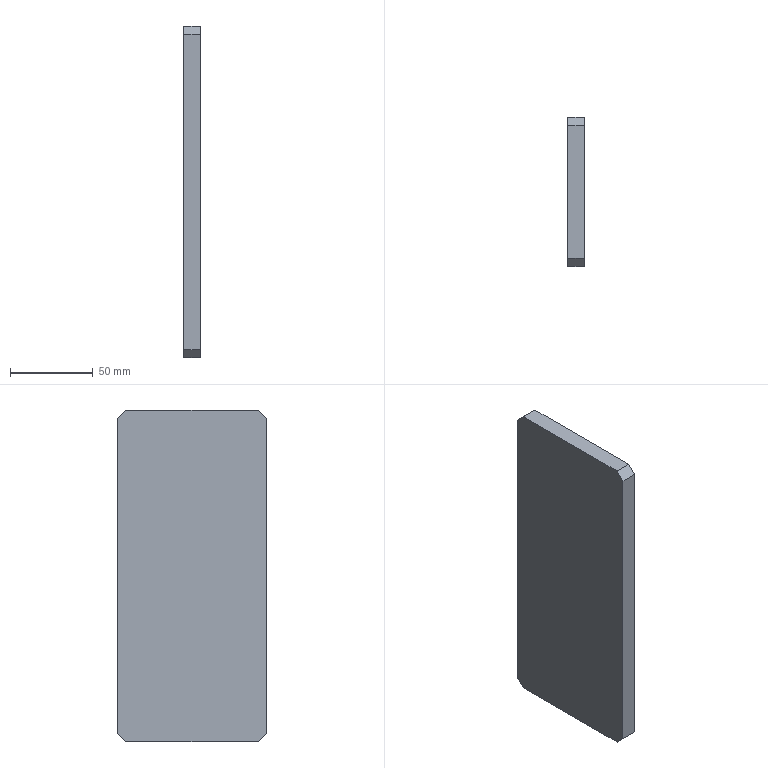Part | SolidWorks | features BaseBody 1 | 1 solid | 10 faces | box 10 x 90 x 200 mm | volume 179500 mm3 | plane 10
STEP:
#1=CARTESIAN_POINT('',(0.,5.,0.));
#2=VERTEX_POINT('',#1);
#3=CARTESIAN_POINT('',(0.,85.,0.));
#4=VERTEX_POINT('',#3);
#5=CARTESIAN_POINT('',(0.,0.,0.));
#6=DIRECTION('',(0.,1.,0.));
#7=VECTOR('',#6,1000.);
#8=LINE('',#5,#7);
#9=EDGE_CURVE('',#2,#4,#8,.T.);
#10=ORIENTED_EDGE('',*,*,#9,.T.);
#11=CARTESIAN_POINT('',(0.,90.,-5.));
#12=VERTEX_POINT('',#11);
#13=CARTESIAN_POINT('',(0.,85.,0.));
#14=DIRECTION('',(0.,0.7071,-0.7071));
#15=VECTOR('',#14,1000.);
#16=LINE('',#13,#15);
#17=EDGE_CURVE('',#4,#12,#16,.T.);
#18=ORIENTED_EDGE('',*,*,#17,.T.);
#19=CARTESIAN_POINT('',(0.,90.,-195.));
#20=VERTEX_POINT('',#19);
#21=CARTESIAN_POINT('',(0.,90.,0.));
#22=DIRECTION('',(0.,0.,-1.));
#23=VECTOR('',#22,1000.);
#24=LINE('',#21,#23);
#25=EDGE_CURVE('',#12,#20,#24,.T.);
#26=ORIENTED_EDGE('',*,*,#25,.T.);
#27=CARTESIAN_POINT('',(0.,85.,-200.));
#28=VERTEX_POINT('',#27);
#29=CARTESIAN_POINT('',(0.,90.,-195.));
#30=DIRECTION('',(0.,-0.7071,-0.7071));
#31=VECTOR('',#30,1000.);
#32=LINE('',#29,#31);
#33=EDGE_CURVE('',#20,#28,#32,.T.);
#34=ORIENTED_EDGE('',*,*,#33,.T.);
#35=CARTESIAN_POINT('',(0.,5.,-200.));
#36=VERTEX_POINT('',#35);
#37=CARTESIAN_POINT('',(0.,0.,-200.));
#38=DIRECTION('',(0.,-1.,0.));
#39=VECTOR('',#38,1000.);
#40=LINE('',#37,#39);
#41=EDGE_CURVE('',#28,#36,#40,.T.);
#42=ORIENTED_EDGE('',*,*,#41,.T.);
#43=CARTESIAN_POINT('',(0.,0.,-195.));
#44=VERTEX_POINT('',#43);
#45=CARTESIAN_POINT('',(0.,5.,-200.));
#46=DIRECTION('',(0.,-0.7071,0.7071));
#47=VECTOR('',#46,1000.);
#48=LINE('',#45,#47);
#49=EDGE_CURVE('',#36,#44,#48,.T.);
#50=ORIENTED_EDGE('',*,*,#49,.T.);
#51=CARTESIAN_POINT('',(0.,0.,-5.));
#52=VERTEX_POINT('',#51);
#53=CARTESIAN_POINT('',(0.,0.,0.));
#54=DIRECTION('',(0.,0.,1.));
#55=VECTOR('',#54,1000.);
#56=LINE('',#53,#55);
#57=EDGE_CURVE('',#44,#52,#56,.T.);
#58=ORIENTED_EDGE('',*,*,#57,.T.);
#59=CARTESIAN_POINT('',(0.,0.,-5.));
#60=DIRECTION('',(0.,0.7071,0.7071));
#61=VECTOR('',#60,1000.);
#62=LINE('',#59,#61);
#63=EDGE_CURVE('',#52,#2,#62,.T.);
#64=ORIENTED_EDGE('',*,*,#63,.T.);
#65=EDGE_LOOP('',(#10,#18,#26,#34,#42,#50,#58,#64));
#66=FACE_OUTER_BOUND('',#65,.T.);
#67=CARTESIAN_POINT('',(0.,0.,0.));
#68=DIRECTION('',(-1.,0.,0.));
#69=DIRECTION('',(0.,0.,1.));
#70=AXIS2_PLACEMENT_3D('',#67,#68,#69);
#71=PLANE('',#70);
#72=ADVANCED_FACE('',(#66),#71,.T.);
#73=CARTESIAN_POINT('',(10.,90.,-5.));
#74=VERTEX_POINT('',#73);
#75=CARTESIAN_POINT('',(10.,90.,-5.));
#76=DIRECTION('',(1.,0.,0.));
#77=VECTOR('',#76,1000.);
#78=LINE('',#75,#77);
#79=EDGE_CURVE('',#12,#74,#78,.T.);
#80=ORIENTED_EDGE('',*,*,#79,.F.);
#81=ORIENTED_EDGE('',*,*,#17,.F.);
#82=CARTESIAN_POINT('',(10.,85.,0.));
#83=VERTEX_POINT('',#82);
#84=CARTESIAN_POINT('',(10.,85.,0.));
#85=DIRECTION('',(-1.,0.,0.));
#86=VECTOR('',#85,1000.);
#87=LINE('',#84,#86);
#88=EDGE_CURVE('',#83,#4,#87,.T.);
#89=ORIENTED_EDGE('',*,*,#88,.F.);
#90=CARTESIAN_POINT('',(10.,85.,0.));
#91=DIRECTION('',(0.,-0.7071,0.7071));
#92=VECTOR('',#91,1000.);
#93=LINE('',#90,#92);
#94=EDGE_CURVE('',#74,#83,#93,.T.);
#95=ORIENTED_EDGE('',*,*,#94,.F.);
#96=EDGE_LOOP('',(#80,#81,#89,#95));
#97=FACE_OUTER_BOUND('',#96,.T.);
#98=CARTESIAN_POINT('',(10.,85.,0.));
#99=DIRECTION('',(0.,-0.7071,-0.7071));
#100=DIRECTION('',(0.,0.7071,-0.7071));
#101=AXIS2_PLACEMENT_3D('',#98,#99,#100);
#102=PLANE('',#101);
#103=ADVANCED_FACE('',(#97),#102,.F.);
#104=CARTESIAN_POINT('',(10.,5.,0.));
#105=VERTEX_POINT('',#104);
#106=CARTESIAN_POINT('',(10.,5.,0.));
#107=DIRECTION('',(-1.,0.,0.));
#108=VECTOR('',#107,1000.);
#109=LINE('',#106,#108);
#110=EDGE_CURVE('',#105,#2,#109,.T.);
#111=ORIENTED_EDGE('',*,*,#110,.F.);
#112=CARTESIAN_POINT('',(10.,0.,0.));
#113=DIRECTION('',(0.,-1.,0.));
#114=VECTOR('',#113,1000.);
#115=LINE('',#112,#114);
#116=EDGE_CURVE('',#83,#105,#115,.T.);
#117=ORIENTED_EDGE('',*,*,#116,.F.);
#118=ORIENTED_EDGE('',*,*,#88,.T.);
#119=ORIENTED_EDGE('',*,*,#9,.F.);
#120=EDGE_LOOP('',(#111,#117,#118,#119));
#121=FACE_OUTER_BOUND('',#120,.T.);
#122=CARTESIAN_POINT('',(10.,0.,0.));
#123=DIRECTION('',(0.,0.,-1.));
#124=DIRECTION('',(0.,1.,0.));
#125=AXIS2_PLACEMENT_3D('',#122,#123,#124);
#126=PLANE('',#125);
#127=ADVANCED_FACE('',(#121),#126,.F.);
#128=ORIENTED_EDGE('',*,*,#110,.T.);
#129=ORIENTED_EDGE('',*,*,#63,.F.);
#130=CARTESIAN_POINT('',(10.,0.,-5.));
#131=VERTEX_POINT('',#130);
#132=CARTESIAN_POINT('',(10.,0.,-5.));
#133=DIRECTION('',(-1.,0.,0.));
#134=VECTOR('',#133,1000.);
#135=LINE('',#132,#134);
#136=EDGE_CURVE('',#131,#52,#135,.T.);
#137=ORIENTED_EDGE('',*,*,#136,.F.);
#138=CARTESIAN_POINT('',(10.,0.,-5.));
#139=DIRECTION('',(0.,-0.7071,-0.7071));
#140=VECTOR('',#139,1000.);
#141=LINE('',#138,#140);
#142=EDGE_CURVE('',#105,#131,#141,.T.);
#143=ORIENTED_EDGE('',*,*,#142,.F.);
#144=EDGE_LOOP('',(#128,#129,#137,#143));
#145=FACE_OUTER_BOUND('',#144,.T.);
#146=CARTESIAN_POINT('',(10.,0.,-5.));
#147=DIRECTION('',(0.,0.7071,-0.7071));
#148=DIRECTION('',(0.,0.7071,0.7071));
#149=AXIS2_PLACEMENT_3D('',#146,#147,#148);
#150=PLANE('',#149);
#151=ADVANCED_FACE('',(#145),#150,.F.);
#152=CARTESIAN_POINT('',(10.,0.,-195.));
#153=VERTEX_POINT('',#152);
#154=CARTESIAN_POINT('',(10.,0.,-195.));
#155=DIRECTION('',(-1.,0.,0.));
#156=VECTOR('',#155,1000.);
#157=LINE('',#154,#156);
#158=EDGE_CURVE('',#153,#44,#157,.T.);
#159=ORIENTED_EDGE('',*,*,#158,.F.);
#160=CARTESIAN_POINT('',(10.,0.,0.));
#161=DIRECTION('',(0.,0.,-1.));
#162=VECTOR('',#161,1000.);
#163=LINE('',#160,#162);
#164=EDGE_CURVE('',#131,#153,#163,.T.);
#165=ORIENTED_EDGE('',*,*,#164,.F.);
#166=ORIENTED_EDGE('',*,*,#136,.T.);
#167=ORIENTED_EDGE('',*,*,#57,.F.);
#168=EDGE_LOOP('',(#159,#165,#166,#167));
#169=FACE_OUTER_BOUND('',#168,.T.);
#170=CARTESIAN_POINT('',(10.,0.,0.));
#171=DIRECTION('',(0.,1.,0.));
#172=DIRECTION('',(0.,0.,1.));
#173=AXIS2_PLACEMENT_3D('',#170,#171,#172);
#174=PLANE('',#173);
#175=ADVANCED_FACE('',(#169),#174,.F.);
#176=ORIENTED_EDGE('',*,*,#158,.T.);
#177=ORIENTED_EDGE('',*,*,#49,.F.);
#178=CARTESIAN_POINT('',(10.,5.,-200.));
#179=VERTEX_POINT('',#178);
#180=CARTESIAN_POINT('',(10.,5.,-200.));
#181=DIRECTION('',(-1.,0.,0.));
#182=VECTOR('',#181,1000.);
#183=LINE('',#180,#182);
#184=EDGE_CURVE('',#179,#36,#183,.T.);
#185=ORIENTED_EDGE('',*,*,#184,.F.);
#186=CARTESIAN_POINT('',(10.,5.,-200.));
#187=DIRECTION('',(0.,0.7071,-0.7071));
#188=VECTOR('',#187,1000.);
#189=LINE('',#186,#188);
#190=EDGE_CURVE('',#153,#179,#189,.T.);
#191=ORIENTED_EDGE('',*,*,#190,.F.);
#192=EDGE_LOOP('',(#176,#177,#185,#191));
#193=FACE_OUTER_BOUND('',#192,.T.);
#194=CARTESIAN_POINT('',(10.,5.,-200.));
#195=DIRECTION('',(0.,0.7071,0.7071));
#196=DIRECTION('',(0.,-0.7071,0.7071));
#197=AXIS2_PLACEMENT_3D('',#194,#195,#196);
#198=PLANE('',#197);
#199=ADVANCED_FACE('',(#193),#198,.F.);
#200=CARTESIAN_POINT('',(10.,85.,-200.));
#201=VERTEX_POINT('',#200);
#202=CARTESIAN_POINT('',(10.,85.,-200.));
#203=DIRECTION('',(-1.,0.,0.));
#204=VECTOR('',#203,1000.);
#205=LINE('',#202,#204);
#206=EDGE_CURVE('',#201,#28,#205,.T.);
#207=ORIENTED_EDGE('',*,*,#206,.F.);
#208=CARTESIAN_POINT('',(10.,0.,-200.));
#209=DIRECTION('',(0.,1.,0.));
#210=VECTOR('',#209,1000.);
#211=LINE('',#208,#210);
#212=EDGE_CURVE('',#179,#201,#211,.T.);
#213=ORIENTED_EDGE('',*,*,#212,.F.);
#214=ORIENTED_EDGE('',*,*,#184,.T.);
#215=ORIENTED_EDGE('',*,*,#41,.F.);
#216=EDGE_LOOP('',(#207,#213,#214,#215));
#217=FACE_OUTER_BOUND('',#216,.T.);
#218=CARTESIAN_POINT('',(10.,0.,-200.));
#219=DIRECTION('',(0.,0.,1.));
#220=DIRECTION('',(0.,-1.,0.));
#221=AXIS2_PLACEMENT_3D('',#218,#219,#220);
#222=PLANE('',#221);
#223=ADVANCED_FACE('',(#217),#222,.F.);
#224=ORIENTED_EDGE('',*,*,#206,.T.);
#225=ORIENTED_EDGE('',*,*,#33,.F.);
#226=CARTESIAN_POINT('',(10.,90.,-195.));
#227=VERTEX_POINT('',#226);
#228=CARTESIAN_POINT('',(10.,90.,-195.));
#229=DIRECTION('',(-1.,0.,0.));
#230=VECTOR('',#229,1000.);
#231=LINE('',#228,#230);
#232=EDGE_CURVE('',#227,#20,#231,.T.);
#233=ORIENTED_EDGE('',*,*,#232,.F.);
#234=CARTESIAN_POINT('',(10.,90.,-195.));
#235=DIRECTION('',(0.,0.7071,0.7071));
#236=VECTOR('',#235,1000.);
#237=LINE('',#234,#236);
#238=EDGE_CURVE('',#201,#227,#237,.T.);
#239=ORIENTED_EDGE('',*,*,#238,.F.);
#240=EDGE_LOOP('',(#224,#225,#233,#239));
#241=FACE_OUTER_BOUND('',#240,.T.);
#242=CARTESIAN_POINT('',(10.,90.,-195.));
#243=DIRECTION('',(0.,-0.7071,0.7071));
#244=DIRECTION('',(0.,-0.7071,-0.7071));
#245=AXIS2_PLACEMENT_3D('',#242,#243,#244);
#246=PLANE('',#245);
#247=ADVANCED_FACE('',(#241),#246,.F.);
#248=ORIENTED_EDGE('',*,*,#232,.T.);
#249=ORIENTED_EDGE('',*,*,#25,.F.);
#250=ORIENTED_EDGE('',*,*,#79,.T.);
#251=CARTESIAN_POINT('',(10.,90.,0.));
#252=DIRECTION('',(0.,0.,1.));
#253=VECTOR('',#252,1000.);
#254=LINE('',#251,#253);
#255=EDGE_CURVE('',#227,#74,#254,.T.);
#256=ORIENTED_EDGE('',*,*,#255,.F.);
#257=EDGE_LOOP('',(#248,#249,#250,#256));
#258=FACE_OUTER_BOUND('',#257,.T.);
#259=CARTESIAN_POINT('',(10.,90.,0.));
#260=DIRECTION('',(0.,-1.,0.));
#261=DIRECTION('',(0.,0.,-1.));
#262=AXIS2_PLACEMENT_3D('',#259,#260,#261);
#263=PLANE('',#262);
#264=ADVANCED_FACE('',(#258),#263,.F.);
#265=ORIENTED_EDGE('',*,*,#238,.T.);
#266=ORIENTED_EDGE('',*,*,#255,.T.);
#267=ORIENTED_EDGE('',*,*,#94,.T.);
#268=ORIENTED_EDGE('',*,*,#116,.T.);
#269=ORIENTED_EDGE('',*,*,#142,.T.);
#270=ORIENTED_EDGE('',*,*,#164,.T.);
#271=ORIENTED_EDGE('',*,*,#190,.T.);
#272=ORIENTED_EDGE('',*,*,#212,.T.);
#273=EDGE_LOOP('',(#265,#266,#267,#268,#269,#270,#271,#272));
#274=FACE_OUTER_BOUND('',#273,.T.);
#275=CARTESIAN_POINT('',(10.,0.,0.));
#276=DIRECTION('',(-1.,0.,0.));
#277=DIRECTION('',(0.,0.,1.));
#278=AXIS2_PLACEMENT_3D('',#275,#276,#277);
#279=PLANE('',#278);
#280=ADVANCED_FACE('',(#274),#279,.F.);
#281=CLOSED_SHELL('',(#72,#103,#127,#151,#175,#199,#223,#247,#264,#280));
#282=MANIFOLD_SOLID_BREP('',#281);
#283=CARTESIAN_POINT('',(0.,0.,0.));
#284=DIRECTION('',(0.,0.,1.));
#285=DIRECTION('',(1.,0.,0.));
#286=AXIS2_PLACEMENT_3D('',#283,#284,#285);
#287=(LENGTH_UNIT()NAMED_UNIT(*)SI_UNIT(.MILLI.,.METRE.));
#288=UNCERTAINTY_MEASURE_WITH_UNIT(LENGTH_MEASURE(0.00001),#287,'','');
#289=(NAMED_UNIT(*)PLANE_ANGLE_UNIT()SI_UNIT($,.RADIAN.));
#290=(NAMED_UNIT(*)SI_UNIT($,.STERADIAN.)SOLID_ANGLE_UNIT());
#291=(GEOMETRIC_REPRESENTATION_CONTEXT(3)GLOBAL_UNCERTAINTY_ASSIGNED_CONTEXT((#288))GLOBAL_UNIT_ASSIGNED_CONTEXT((#287,#289,#290))REPRESENTATION_CONTEXT('',''));
#292=ADVANCED_BREP_SHAPE_REPRESENTATION('',(#282,#286),#291);